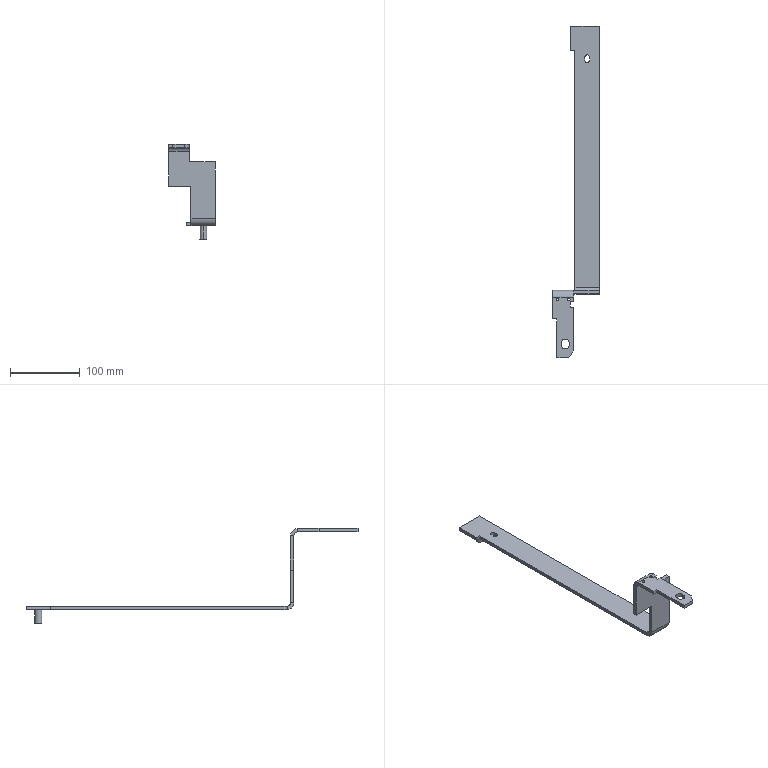Part | STEP file | 64562487 | 1 solid | 50 faces | box 67.1 x 477 x 136.5 mm | volume 104074 mm3 | plane 36 | cylinder 14 | commonest cylinder face diameters 4 x4 10 x4 7 x2 12 x2 20 x2